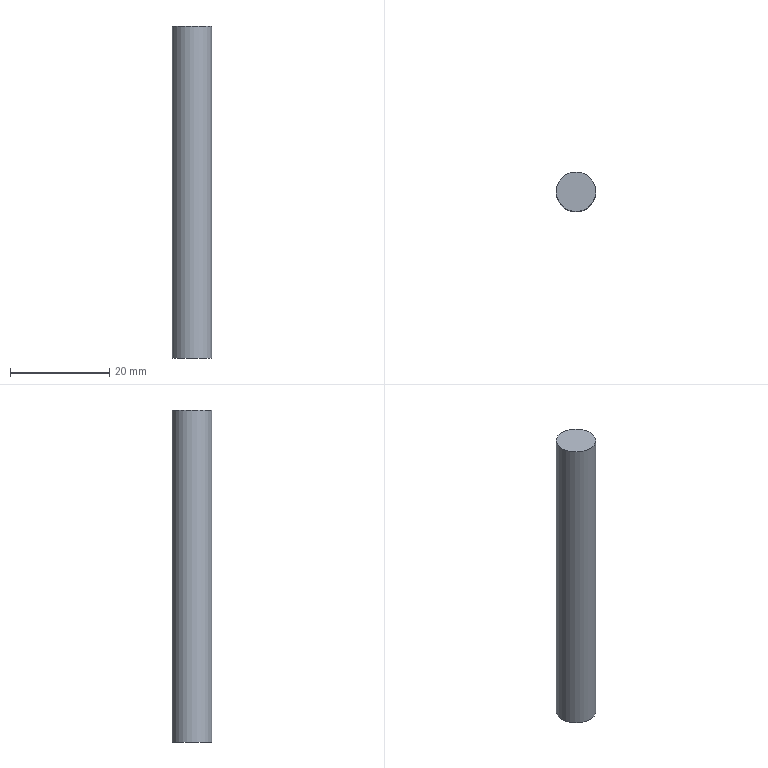Part | STEP file | Tube feed_id938_x_t | 1 solid | 6 faces | box 8 x 8 x 67 mm | volume 3084 mm3 | plane 2 | cylinder 2 | cone 2 | commonest cylinder face diameters 4.2 x1 8 x1
STEP:
#1=CARTESIAN_POINT('',(0.,0.,0.));
#2=DIRECTION('',(0.,0.,1.));
#3=DIRECTION('',(1.,0.,0.));
#4=AXIS2_PLACEMENT_3D('',#1,#2,#3);
#5=CARTESIAN_POINT('',(-145.,20.056,-9.4));
#6=VERTEX_POINT('',#5);
#7=CARTESIAN_POINT('',(-149.,20.056,-9.4));
#8=DIRECTION('',(0.,0.,-1.));
#9=DIRECTION('',(1.,0.,0.));
#10=AXIS2_PLACEMENT_3D('',#7,#8,#9);
#11=CIRCLE('',#10,4.);
#12=CARTESIAN_POINT('',(-149.,20.056,-9.4));
#13=DIRECTION('',(0.,0.,1.));
#14=DIRECTION('',(1.,0.,0.));
#15=AXIS2_PLACEMENT_3D('',#12,#13,#14);
#16=PLANE('',#15);
#17=CARTESIAN_POINT('',(4.,0.));
#18=CARTESIAN_POINT('',(4.,-6.928));
#19=CARTESIAN_POINT('',(-2.,-3.464));
#20=CARTESIAN_POINT('',(-8.,0.));
#21=CARTESIAN_POINT('',(-2.,3.464));
#22=CARTESIAN_POINT('',(4.,6.928));
#23=CARTESIAN_POINT('',(4.,0.));
#24=(BOUNDED_CURVE()B_SPLINE_CURVE(2,(#17,#18,#19,#20,#21,#22,#23),.UNSPECIFIED.,.T.,.F.)B_SPLINE_CURVE_WITH_KNOTS((1,2,2,2,2,1),(-2.094,0.,2.094,4.189,6.283,8.378),.UNSPECIFIED.)CURVE()GEOMETRIC_REPRESENTATION_ITEM()RATIONAL_B_SPLINE_CURVE((1.,0.5,1.,0.5,1.,0.5,1.))REPRESENTATION_ITEM(''));
#25=(GEOMETRIC_REPRESENTATION_CONTEXT(2)PARAMETRIC_REPRESENTATION_CONTEXT()REPRESENTATION_CONTEXT('',''));
#26=DEFINITIONAL_REPRESENTATION('',(#24),#25);
#27=PCURVE('',#16,#26);
#28=CARTESIAN_POINT('',(-149.,20.056,-76.4));
#29=DIRECTION('',(0.,0.,1.));
#30=DIRECTION('',(1.,0.,0.));
#31=AXIS2_PLACEMENT_3D('',#28,#29,#30);
#32=CYLINDRICAL_SURFACE('',#31,4.);
#33=CARTESIAN_POINT('',(6.283,67.));
#34=DIRECTION('',(-1.,0.));
#35=VECTOR('',#34,1.);
#36=LINE('',#33,#35);
#37=(GEOMETRIC_REPRESENTATION_CONTEXT(2)PARAMETRIC_REPRESENTATION_CONTEXT()REPRESENTATION_CONTEXT('',''));
#38=DEFINITIONAL_REPRESENTATION('',(#36),#37);
#39=PCURVE('',#32,#38);
#40=SURFACE_CURVE('',#11,(#27,#39),.PCURVE_S1.);
#41=EDGE_CURVE('',#6,#6,#40,.T.);
#42=ORIENTED_EDGE('',*,*,#41,.F.);
#43=EDGE_LOOP('',(#42));
#44=FACE_BOUND('',#43,.T.);
#45=ADVANCED_FACE('',(#44),#16,.T.);
#46=CARTESIAN_POINT('',(-151.5,20.056,-76.4));
#47=VERTEX_POINT('',#46);
#48=CARTESIAN_POINT('',(-149.,20.056,-76.4));
#49=DIRECTION('',(0.,0.,1.));
#50=DIRECTION('',(-1.,0.,0.));
#51=AXIS2_PLACEMENT_3D('',#48,#49,#50);
#52=CIRCLE('',#51,2.5);
#53=CARTESIAN_POINT('',(-149.,20.056,-76.4));
#54=DIRECTION('',(0.,0.,-1.));
#55=DIRECTION('',(-1.,0.,0.));
#56=AXIS2_PLACEMENT_3D('',#53,#54,#55);
#57=PLANE('',#56);
#58=CARTESIAN_POINT('',(2.5,0.));
#59=CARTESIAN_POINT('',(2.5,-4.33));
#60=CARTESIAN_POINT('',(-1.25,-2.165));
#61=CARTESIAN_POINT('',(-5.,0.));
#62=CARTESIAN_POINT('',(-1.25,2.165));
#63=CARTESIAN_POINT('',(2.5,4.33));
#64=CARTESIAN_POINT('',(2.5,0.));
#65=(BOUNDED_CURVE()B_SPLINE_CURVE(2,(#58,#59,#60,#61,#62,#63,#64),.UNSPECIFIED.,.T.,.F.)B_SPLINE_CURVE_WITH_KNOTS((1,2,2,2,2,1),(-2.094,0.,2.094,4.189,6.283,8.378),.UNSPECIFIED.)CURVE()GEOMETRIC_REPRESENTATION_ITEM()RATIONAL_B_SPLINE_CURVE((1.,0.5,1.,0.5,1.,0.5,1.))REPRESENTATION_ITEM(''));
#66=(GEOMETRIC_REPRESENTATION_CONTEXT(2)PARAMETRIC_REPRESENTATION_CONTEXT()REPRESENTATION_CONTEXT('',''));
#67=DEFINITIONAL_REPRESENTATION('',(#65),#66);
#68=PCURVE('',#57,#67);
#69=CARTESIAN_POINT('',(-149.,20.056,-76.4));
#70=DIRECTION('',(0.,0.,-1.));
#71=DIRECTION('',(-1.,0.,0.));
#72=AXIS2_PLACEMENT_3D('',#69,#70,#71);
#73=CONICAL_SURFACE('',#72,2.5,0.7854);
#74=CARTESIAN_POINT('',(6.283,0.));
#75=DIRECTION('',(-1.,0.));
#76=VECTOR('',#75,1.);
#77=LINE('',#74,#76);
#78=(GEOMETRIC_REPRESENTATION_CONTEXT(2)PARAMETRIC_REPRESENTATION_CONTEXT()REPRESENTATION_CONTEXT('',''));
#79=DEFINITIONAL_REPRESENTATION('',(#77),#78);
#80=PCURVE('',#73,#79);
#81=SURFACE_CURVE('',#52,(#68,#80),.PCURVE_S1.);
#82=EDGE_CURVE('',#47,#47,#81,.T.);
#83=ORIENTED_EDGE('',*,*,#82,.T.);
#84=EDGE_LOOP('',(#83));
#85=FACE_BOUND('',#84,.T.);
#86=CARTESIAN_POINT('',(-145.,20.056,-76.4));
#87=VERTEX_POINT('',#86);
#88=CARTESIAN_POINT('',(-149.,20.056,-76.4));
#89=DIRECTION('',(0.,0.,1.));
#90=DIRECTION('',(1.,0.,0.));
#91=AXIS2_PLACEMENT_3D('',#88,#89,#90);
#92=CIRCLE('',#91,4.);
#93=CARTESIAN_POINT('',(-4.,0.));
#94=CARTESIAN_POINT('',(-4.,6.928));
#95=CARTESIAN_POINT('',(2.,3.464));
#96=CARTESIAN_POINT('',(8.,0.));
#97=CARTESIAN_POINT('',(2.,-3.464));
#98=CARTESIAN_POINT('',(-4.,-6.928));
#99=CARTESIAN_POINT('',(-4.,0.));
#100=(BOUNDED_CURVE()B_SPLINE_CURVE(2,(#93,#94,#95,#96,#97,#98,#99),.UNSPECIFIED.,.T.,.F.)B_SPLINE_CURVE_WITH_KNOTS((1,2,2,2,2,1),(-2.094,0.,2.094,4.189,6.283,8.378),.UNSPECIFIED.)CURVE()GEOMETRIC_REPRESENTATION_ITEM()RATIONAL_B_SPLINE_CURVE((1.,0.5,1.,0.5,1.,0.5,1.))REPRESENTATION_ITEM(''));
#101=(GEOMETRIC_REPRESENTATION_CONTEXT(2)PARAMETRIC_REPRESENTATION_CONTEXT()REPRESENTATION_CONTEXT('',''));
#102=DEFINITIONAL_REPRESENTATION('',(#100),#101);
#103=PCURVE('',#57,#102);
#104=CARTESIAN_POINT('',(0.,0.));
#105=DIRECTION('',(1.,0.));
#106=VECTOR('',#105,1.);
#107=LINE('',#104,#106);
#108=(GEOMETRIC_REPRESENTATION_CONTEXT(2)PARAMETRIC_REPRESENTATION_CONTEXT()REPRESENTATION_CONTEXT('',''));
#109=DEFINITIONAL_REPRESENTATION('',(#107),#108);
#110=PCURVE('',#32,#109);
#111=SURFACE_CURVE('',#92,(#103,#110),.PCURVE_S1.);
#112=EDGE_CURVE('',#87,#87,#111,.T.);
#113=ORIENTED_EDGE('',*,*,#112,.F.);
#114=EDGE_LOOP('',(#113));
#115=FACE_BOUND('',#114,.T.);
#116=ADVANCED_FACE('',(#85,#115),#57,.T.);
#117=ORIENTED_EDGE('',*,*,#41,.T.);
#118=CARTESIAN_POINT('',(-145.,20.056,-76.4));
#119=CARTESIAN_POINT('',(-145.,20.056,-9.4));
#120=B_SPLINE_CURVE_WITH_KNOTS('',1,(#118,#119),.UNSPECIFIED.,.F.,.F.,(2,2),(0.,67.),.PIECEWISE_BEZIER_KNOTS.);
#121=CARTESIAN_POINT('',(0.,0.));
#122=DIRECTION('',(0.,1.));
#123=VECTOR('',#122,1.);
#124=LINE('',#121,#123);
#125=(GEOMETRIC_REPRESENTATION_CONTEXT(2)PARAMETRIC_REPRESENTATION_CONTEXT()REPRESENTATION_CONTEXT('',''));
#126=DEFINITIONAL_REPRESENTATION('',(#124),#125);
#127=PCURVE('',#32,#126);
#128=CARTESIAN_POINT('',(6.283,0.));
#129=DIRECTION('',(0.,1.));
#130=VECTOR('',#129,1.);
#131=LINE('',#128,#130);
#132=(GEOMETRIC_REPRESENTATION_CONTEXT(2)PARAMETRIC_REPRESENTATION_CONTEXT()REPRESENTATION_CONTEXT('',''));
#133=DEFINITIONAL_REPRESENTATION('',(#131),#132);
#134=PCURVE('',#32,#133);
#135=SEAM_CURVE('',#120,(#127,#134),.PCURVE_S1.);
#136=EDGE_CURVE('',#87,#6,#135,.T.);
#137=ORIENTED_EDGE('',*,*,#136,.F.);
#138=ORIENTED_EDGE('',*,*,#112,.T.);
#139=ORIENTED_EDGE('',*,*,#136,.T.);
#140=EDGE_LOOP('',(#117,#137,#138,#139));
#141=FACE_BOUND('',#140,.T.);
#142=ADVANCED_FACE('',(#141),#32,.T.);
#143=CARTESIAN_POINT('',(-151.1,20.056,-56.4));
#144=VERTEX_POINT('',#143);
#145=CARTESIAN_POINT('',(-146.9,20.056,-56.4));
#146=VERTEX_POINT('',#145);
#147=CARTESIAN_POINT('',(-149.,20.056,-56.4));
#148=DIRECTION('',(0.,0.,-1.));
#149=DIRECTION('',(1.,0.,0.));
#150=AXIS2_PLACEMENT_3D('',#147,#148,#149);
#151=CIRCLE('',#150,2.1);
#152=CARTESIAN_POINT('',(-149.,20.056,-56.4));
#153=DIRECTION('',(0.,0.,-1.));
#154=DIRECTION('',(-1.,0.,0.));
#155=AXIS2_PLACEMENT_3D('',#152,#153,#154);
#156=CONICAL_SURFACE('',#155,2.1,1.03);
#157=CARTESIAN_POINT('',(-3.142,0.));
#158=DIRECTION('',(1.,0.));
#159=VECTOR('',#158,1.);
#160=LINE('',#157,#159);
#161=(GEOMETRIC_REPRESENTATION_CONTEXT(2)PARAMETRIC_REPRESENTATION_CONTEXT()REPRESENTATION_CONTEXT('',''));
#162=DEFINITIONAL_REPRESENTATION('',(#160),#161);
#163=PCURVE('',#156,#162);
#164=CARTESIAN_POINT('',(-149.,20.056,-76.4));
#165=DIRECTION('',(0.,0.,1.));
#166=DIRECTION('',(1.,0.,0.));
#167=AXIS2_PLACEMENT_3D('',#164,#165,#166);
#168=CYLINDRICAL_SURFACE('',#167,2.1);
#169=CARTESIAN_POINT('',(12.566,20.));
#170=DIRECTION('',(-1.,0.));
#171=VECTOR('',#170,1.);
#172=LINE('',#169,#171);
#173=(GEOMETRIC_REPRESENTATION_CONTEXT(2)PARAMETRIC_REPRESENTATION_CONTEXT()REPRESENTATION_CONTEXT('',''));
#174=DEFINITIONAL_REPRESENTATION('',(#172),#173);
#175=PCURVE('',#168,#174);
#176=SURFACE_CURVE('',#151,(#163,#175),.PCURVE_S1.);
#177=EDGE_CURVE('',#144,#146,#176,.T.);
#178=ORIENTED_EDGE('',*,*,#177,.F.);
#179=CARTESIAN_POINT('',(-149.,20.056,-55.138));
#180=VERTEX_POINT('',#179);
#181=CARTESIAN_POINT('',(-149.,20.056,-55.138));
#182=CARTESIAN_POINT('',(-151.1,20.056,-56.4));
#183=B_SPLINE_CURVE_WITH_KNOTS('',1,(#181,#182),.UNSPECIFIED.,.F.,.F.,(2,2),(-2.45,0.),.PIECEWISE_BEZIER_KNOTS.);
#184=CARTESIAN_POINT('',(0.,0.));
#185=DIRECTION('',(0.,1.));
#186=VECTOR('',#185,1.);
#187=LINE('',#184,#186);
#188=(GEOMETRIC_REPRESENTATION_CONTEXT(2)PARAMETRIC_REPRESENTATION_CONTEXT()REPRESENTATION_CONTEXT('',''));
#189=DEFINITIONAL_REPRESENTATION('',(#187),#188);
#190=PCURVE('',#156,#189);
#191=CARTESIAN_POINT('',(6.283,0.));
#192=DIRECTION('',(0.,1.));
#193=VECTOR('',#192,1.);
#194=LINE('',#191,#193);
#195=(GEOMETRIC_REPRESENTATION_CONTEXT(2)PARAMETRIC_REPRESENTATION_CONTEXT()REPRESENTATION_CONTEXT('',''));
#196=DEFINITIONAL_REPRESENTATION('',(#194),#195);
#197=PCURVE('',#156,#196);
#198=SEAM_CURVE('',#183,(#190,#197),.PCURVE_S1.);
#199=EDGE_CURVE('',#180,#144,#198,.T.);
#200=ORIENTED_EDGE('',*,*,#199,.F.);
#201=ORIENTED_EDGE('',*,*,#199,.T.);
#202=CARTESIAN_POINT('',(-149.,20.056,-56.4));
#203=DIRECTION('',(0.,0.,-1.));
#204=DIRECTION('',(1.,0.,0.));
#205=AXIS2_PLACEMENT_3D('',#202,#203,#204);
#206=CIRCLE('',#205,2.1);
#207=CARTESIAN_POINT('',(3.142,0.));
#208=DIRECTION('',(1.,0.));
#209=VECTOR('',#208,1.);
#210=LINE('',#207,#209);
#211=(GEOMETRIC_REPRESENTATION_CONTEXT(2)PARAMETRIC_REPRESENTATION_CONTEXT()REPRESENTATION_CONTEXT('',''));
#212=DEFINITIONAL_REPRESENTATION('',(#210),#211);
#213=PCURVE('',#156,#212);
#214=CARTESIAN_POINT('',(6.283,20.));
#215=DIRECTION('',(-1.,0.));
#216=VECTOR('',#215,1.);
#217=LINE('',#214,#216);
#218=(GEOMETRIC_REPRESENTATION_CONTEXT(2)PARAMETRIC_REPRESENTATION_CONTEXT()REPRESENTATION_CONTEXT('',''));
#219=DEFINITIONAL_REPRESENTATION('',(#217),#218);
#220=PCURVE('',#168,#219);
#221=SURFACE_CURVE('',#206,(#213,#220),.PCURVE_S1.);
#222=EDGE_CURVE('',#146,#144,#221,.T.);
#223=ORIENTED_EDGE('',*,*,#222,.F.);
#224=EDGE_LOOP('',(#178,#200,#201,#223));
#225=FACE_BOUND('',#224,.F.);
#226=ADVANCED_FACE('',(#225),#156,.F.);
#227=CARTESIAN_POINT('',(-151.1,20.056,-76.));
#228=VERTEX_POINT('',#227);
#229=CARTESIAN_POINT('',(-149.,20.056,-76.));
#230=DIRECTION('',(0.,0.,-1.));
#231=DIRECTION('',(-1.,0.,0.));
#232=AXIS2_PLACEMENT_3D('',#229,#230,#231);
#233=CIRCLE('',#232,2.1);
#234=CARTESIAN_POINT('',(9.425,0.4));
#235=DIRECTION('',(-1.,0.));
#236=VECTOR('',#235,1.);
#237=LINE('',#234,#236);
#238=(GEOMETRIC_REPRESENTATION_CONTEXT(2)PARAMETRIC_REPRESENTATION_CONTEXT()REPRESENTATION_CONTEXT('',''));
#239=DEFINITIONAL_REPRESENTATION('',(#237),#238);
#240=PCURVE('',#168,#239);
#241=CARTESIAN_POINT('',(0.,-0.4));
#242=DIRECTION('',(1.,0.));
#243=VECTOR('',#242,1.);
#244=LINE('',#241,#243);
#245=(GEOMETRIC_REPRESENTATION_CONTEXT(2)PARAMETRIC_REPRESENTATION_CONTEXT()REPRESENTATION_CONTEXT('',''));
#246=DEFINITIONAL_REPRESENTATION('',(#244),#245);
#247=PCURVE('',#73,#246);
#248=SURFACE_CURVE('',#233,(#240,#247),.PCURVE_S1.);
#249=EDGE_CURVE('',#228,#228,#248,.T.);
#250=ORIENTED_EDGE('',*,*,#249,.F.);
#251=CARTESIAN_POINT('',(-151.1,20.056,-76.));
#252=CARTESIAN_POINT('',(-151.1,20.056,-56.4));
#253=B_SPLINE_CURVE_WITH_KNOTS('',1,(#251,#252),.UNSPECIFIED.,.F.,.F.,(2,2),(0.4,20.),.PIECEWISE_BEZIER_KNOTS.);
#254=CARTESIAN_POINT('',(9.425,0.));
#255=DIRECTION('',(0.,1.));
#256=VECTOR('',#255,1.);
#257=LINE('',#254,#256);
#258=(GEOMETRIC_REPRESENTATION_CONTEXT(2)PARAMETRIC_REPRESENTATION_CONTEXT()REPRESENTATION_CONTEXT('',''));
#259=DEFINITIONAL_REPRESENTATION('',(#257),#258);
#260=PCURVE('',#168,#259);
#261=CARTESIAN_POINT('',(3.142,0.));
#262=DIRECTION('',(0.,1.));
#263=VECTOR('',#262,1.);
#264=LINE('',#261,#263);
#265=(GEOMETRIC_REPRESENTATION_CONTEXT(2)PARAMETRIC_REPRESENTATION_CONTEXT()REPRESENTATION_CONTEXT('',''));
#266=DEFINITIONAL_REPRESENTATION('',(#264),#265);
#267=PCURVE('',#168,#266);
#268=SEAM_CURVE('',#253,(#260,#267),.PCURVE_S1.);
#269=EDGE_CURVE('',#228,#144,#268,.T.);
#270=ORIENTED_EDGE('',*,*,#269,.T.);
#271=ORIENTED_EDGE('',*,*,#177,.T.);
#272=ORIENTED_EDGE('',*,*,#222,.T.);
#273=ORIENTED_EDGE('',*,*,#269,.F.);
#274=EDGE_LOOP('',(#250,#270,#271,#272,#273));
#275=FACE_BOUND('',#274,.F.);
#276=ADVANCED_FACE('',(#275),#168,.F.);
#277=ORIENTED_EDGE('',*,*,#249,.T.);
#278=CARTESIAN_POINT('',(-151.1,20.056,-76.));
#279=CARTESIAN_POINT('',(-151.5,20.056,-76.4));
#280=B_SPLINE_CURVE_WITH_KNOTS('',1,(#278,#279),.UNSPECIFIED.,.F.,.F.,(2,2),(-0.5657,0.),.PIECEWISE_BEZIER_KNOTS.);
#281=CARTESIAN_POINT('',(6.283,0.));
#282=DIRECTION('',(0.,1.));
#283=VECTOR('',#282,1.);
#284=LINE('',#281,#283);
#285=(GEOMETRIC_REPRESENTATION_CONTEXT(2)PARAMETRIC_REPRESENTATION_CONTEXT()REPRESENTATION_CONTEXT('',''));
#286=DEFINITIONAL_REPRESENTATION('',(#284),#285);
#287=PCURVE('',#73,#286);
#288=CARTESIAN_POINT('',(0.,0.));
#289=DIRECTION('',(0.,1.));
#290=VECTOR('',#289,1.);
#291=LINE('',#288,#290);
#292=(GEOMETRIC_REPRESENTATION_CONTEXT(2)PARAMETRIC_REPRESENTATION_CONTEXT()REPRESENTATION_CONTEXT('',''));
#293=DEFINITIONAL_REPRESENTATION('',(#291),#292);
#294=PCURVE('',#73,#293);
#295=SEAM_CURVE('',#280,(#287,#294),.PCURVE_S1.);
#296=EDGE_CURVE('',#228,#47,#295,.T.);
#297=ORIENTED_EDGE('',*,*,#296,.T.);
#298=ORIENTED_EDGE('',*,*,#82,.T.);
#299=ORIENTED_EDGE('',*,*,#296,.F.);
#300=EDGE_LOOP('',(#277,#297,#298,#299));
#301=FACE_BOUND('',#300,.F.);
#302=ADVANCED_FACE('',(#301),#73,.F.);
#303=CLOSED_SHELL('',(#45,#116,#142,#226,#276,#302));
#304=MANIFOLD_SOLID_BREP('',#303);
#305=(LENGTH_UNIT()NAMED_UNIT(*)SI_UNIT(.MILLI.,.METRE.));
#306=UNCERTAINTY_MEASURE_WITH_UNIT(LENGTH_MEASURE(0.00001),#305,'','');
#307=(NAMED_UNIT(*)PLANE_ANGLE_UNIT()SI_UNIT($,.RADIAN.));
#308=(NAMED_UNIT(*)SI_UNIT($,.STERADIAN.)SOLID_ANGLE_UNIT());
#309=(GEOMETRIC_REPRESENTATION_CONTEXT(3)GLOBAL_UNCERTAINTY_ASSIGNED_CONTEXT((#306))GLOBAL_UNIT_ASSIGNED_CONTEXT((#305,#307,#308))REPRESENTATION_CONTEXT('',''));
#310=ADVANCED_BREP_SHAPE_REPRESENTATION('',(#4,#304),#309);